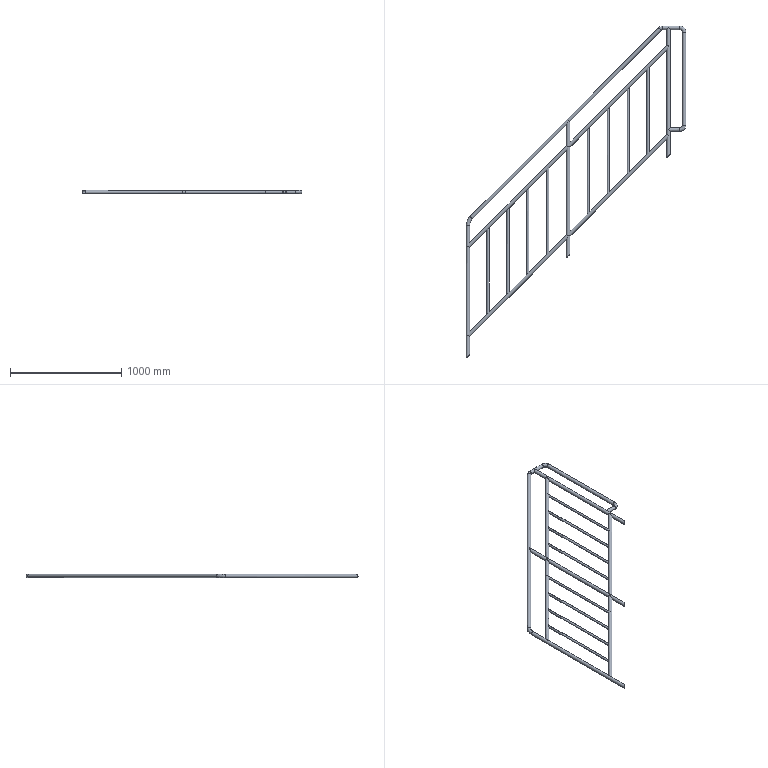Part | STEP file | PN_0050 stair guardrail B_Default<As Machined> | 23 solids | 92 faces | box 1972 x 2980 x 32 mm | volume 2990354 mm3 | cylinder 61 | plane 23 | torus 8 | commonest cylinder face diameters 32 x34 28 x11 16 x8 20 x8